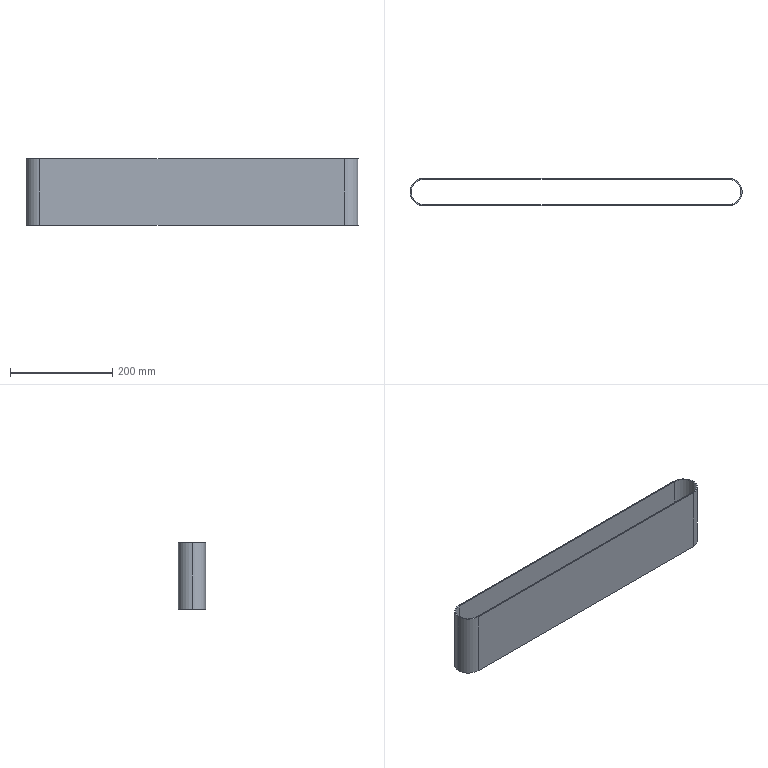Part | STEP file | Light green PVC conveyor belt 1346x129x2mm thick_antistatic | 1 solid | 12 faces | box 648.5 x 54 x 129 mm | volume 348910 mm3 | cylinder 6 | plane 6 | commonest cylinder face diameters 50 x3 54 x3
STEP:
#1=CARTESIAN_POINT('',(0.,0.,0.));
#2=DIRECTION('',(0.,0.,1.));
#3=DIRECTION('',(1.,0.,0.));
#4=AXIS2_PLACEMENT_3D('',#1,#2,#3);
#5=CARTESIAN_POINT('',(-297.25,25.,64.5));
#6=VERTEX_POINT('',#5);
#7=CARTESIAN_POINT('',(-297.25,25.,-64.5));
#8=VERTEX_POINT('',#7);
#9=CARTESIAN_POINT('',(-297.25,25.,64.5));
#10=DIRECTION('',(0.,0.,-1.));
#11=VECTOR('',#10,1.);
#12=LINE('',#9,#11);
#13=CARTESIAN_POINT('',(-297.25,0.,64.5));
#14=DIRECTION('',(0.,0.,-1.));
#15=DIRECTION('',(-1.,0.,0.));
#16=AXIS2_PLACEMENT_3D('',#13,#14,#15);
#17=CYLINDRICAL_SURFACE('',#16,25.);
#18=CARTESIAN_POINT('',(1.571,0.));
#19=DIRECTION('',(0.,1.));
#20=VECTOR('',#19,1.);
#21=LINE('',#18,#20);
#22=(GEOMETRIC_REPRESENTATION_CONTEXT(2)PARAMETRIC_REPRESENTATION_CONTEXT()REPRESENTATION_CONTEXT('',''));
#23=DEFINITIONAL_REPRESENTATION('',(#21),#22);
#24=PCURVE('',#17,#23);
#25=CARTESIAN_POINT('',(-297.25,25.,64.5));
#26=DIRECTION('',(0.,-1.,0.));
#27=DIRECTION('',(0.,0.,-1.));
#28=AXIS2_PLACEMENT_3D('',#25,#26,#27);
#29=PLANE('',#28);
#30=CARTESIAN_POINT('',(0.,0.));
#31=DIRECTION('',(1.,0.));
#32=VECTOR('',#31,1.);
#33=LINE('',#30,#32);
#34=(GEOMETRIC_REPRESENTATION_CONTEXT(2)PARAMETRIC_REPRESENTATION_CONTEXT()REPRESENTATION_CONTEXT('',''));
#35=DEFINITIONAL_REPRESENTATION('',(#33),#34);
#36=PCURVE('',#29,#35);
#37=SURFACE_CURVE('',#12,(#24,#36),.PCURVE_S1.);
#38=EDGE_CURVE('',#6,#8,#37,.T.);
#39=ORIENTED_EDGE('',*,*,#38,.T.);
#40=CARTESIAN_POINT('',(-322.25,0.,-64.5));
#41=VERTEX_POINT('',#40);
#42=CARTESIAN_POINT('',(-297.25,0.,-64.5));
#43=DIRECTION('',(0.,0.,1.));
#44=DIRECTION('',(1.,0.,0.));
#45=AXIS2_PLACEMENT_3D('',#42,#43,#44);
#46=CIRCLE('',#45,25.);
#47=CARTESIAN_POINT('',(3.142,129.));
#48=DIRECTION('',(-1.,0.));
#49=VECTOR('',#48,1.);
#50=LINE('',#47,#49);
#51=(GEOMETRIC_REPRESENTATION_CONTEXT(2)PARAMETRIC_REPRESENTATION_CONTEXT()REPRESENTATION_CONTEXT('',''));
#52=DEFINITIONAL_REPRESENTATION('',(#50),#51);
#53=PCURVE('',#17,#52);
#54=CARTESIAN_POINT('',(-297.25,0.,-64.5));
#55=DIRECTION('',(0.,0.,1.));
#56=DIRECTION('',(1.,0.,0.));
#57=AXIS2_PLACEMENT_3D('',#54,#55,#56);
#58=PLANE('',#57);
#59=CARTESIAN_POINT('',(0.,0.));
#60=DIRECTION('',(1.,0.));
#61=AXIS2_PLACEMENT_2D('',#59,#60);
#62=CIRCLE('',#61,25.);
#63=(GEOMETRIC_REPRESENTATION_CONTEXT(2)PARAMETRIC_REPRESENTATION_CONTEXT()REPRESENTATION_CONTEXT('',''));
#64=DEFINITIONAL_REPRESENTATION('',(#62),#63);
#65=PCURVE('',#58,#64);
#66=SURFACE_CURVE('',#46,(#53,#65),.PCURVE_S1.);
#67=EDGE_CURVE('',#8,#41,#66,.T.);
#68=ORIENTED_EDGE('',*,*,#67,.T.);
#69=CARTESIAN_POINT('',(-322.25,0.,64.5));
#70=VERTEX_POINT('',#69);
#71=CARTESIAN_POINT('',(-322.25,0.,64.5));
#72=DIRECTION('',(0.,0.,-1.));
#73=VECTOR('',#72,1.);
#74=LINE('',#71,#73);
#75=CARTESIAN_POINT('',(0.,0.));
#76=DIRECTION('',(0.,1.));
#77=VECTOR('',#76,1.);
#78=LINE('',#75,#77);
#79=(GEOMETRIC_REPRESENTATION_CONTEXT(2)PARAMETRIC_REPRESENTATION_CONTEXT()REPRESENTATION_CONTEXT('',''));
#80=DEFINITIONAL_REPRESENTATION('',(#78),#79);
#81=PCURVE('',#17,#80);
#82=CARTESIAN_POINT('',(-297.25,0.,64.5));
#83=DIRECTION('',(0.,0.,-1.));
#84=DIRECTION('',(-1.,0.,0.));
#85=AXIS2_PLACEMENT_3D('',#82,#83,#84);
#86=CYLINDRICAL_SURFACE('',#85,25.);
#87=CARTESIAN_POINT('',(6.283,0.));
#88=DIRECTION('',(0.,1.));
#89=VECTOR('',#88,1.);
#90=LINE('',#87,#89);
#91=(GEOMETRIC_REPRESENTATION_CONTEXT(2)PARAMETRIC_REPRESENTATION_CONTEXT()REPRESENTATION_CONTEXT('',''));
#92=DEFINITIONAL_REPRESENTATION('',(#90),#91);
#93=PCURVE('',#86,#92);
#94=SURFACE_CURVE('',#74,(#81,#93),.PCURVE_S1.);
#95=EDGE_CURVE('',#70,#41,#94,.T.);
#96=ORIENTED_EDGE('',*,*,#95,.F.);
#97=CARTESIAN_POINT('',(-297.25,0.,64.5));
#98=DIRECTION('',(0.,0.,1.));
#99=DIRECTION('',(1.,0.,0.));
#100=AXIS2_PLACEMENT_3D('',#97,#98,#99);
#101=CIRCLE('',#100,25.);
#102=CARTESIAN_POINT('',(3.142,0.));
#103=DIRECTION('',(-1.,0.));
#104=VECTOR('',#103,1.);
#105=LINE('',#102,#104);
#106=(GEOMETRIC_REPRESENTATION_CONTEXT(2)PARAMETRIC_REPRESENTATION_CONTEXT()REPRESENTATION_CONTEXT('',''));
#107=DEFINITIONAL_REPRESENTATION('',(#105),#106);
#108=PCURVE('',#17,#107);
#109=CARTESIAN_POINT('',(-297.25,0.,64.5));
#110=DIRECTION('',(0.,0.,1.));
#111=DIRECTION('',(1.,0.,0.));
#112=AXIS2_PLACEMENT_3D('',#109,#110,#111);
#113=PLANE('',#112);
#114=CARTESIAN_POINT('',(0.,0.));
#115=DIRECTION('',(1.,0.));
#116=AXIS2_PLACEMENT_2D('',#114,#115);
#117=CIRCLE('',#116,25.);
#118=(GEOMETRIC_REPRESENTATION_CONTEXT(2)PARAMETRIC_REPRESENTATION_CONTEXT()REPRESENTATION_CONTEXT('',''));
#119=DEFINITIONAL_REPRESENTATION('',(#117),#118);
#120=PCURVE('',#113,#119);
#121=SURFACE_CURVE('',#101,(#108,#120),.PCURVE_S1.);
#122=EDGE_CURVE('',#6,#70,#121,.T.);
#123=ORIENTED_EDGE('',*,*,#122,.F.);
#124=EDGE_LOOP('',(#39,#68,#96,#123));
#125=FACE_BOUND('',#124,.F.);
#126=ADVANCED_FACE('',(#125),#17,.F.);
#127=CARTESIAN_POINT('',(-324.25,0.,64.5));
#128=VERTEX_POINT('',#127);
#129=CARTESIAN_POINT('',(-297.25,-27.,64.5));
#130=VERTEX_POINT('',#129);
#131=CARTESIAN_POINT('',(-297.25,0.,64.5));
#132=DIRECTION('',(0.,0.,1.));
#133=DIRECTION('',(1.,0.,0.));
#134=AXIS2_PLACEMENT_3D('',#131,#132,#133);
#135=CIRCLE('',#134,27.);
#136=CARTESIAN_POINT('',(-297.25,0.,64.5));
#137=DIRECTION('',(0.,0.,-1.));
#138=DIRECTION('',(-1.,0.,0.));
#139=AXIS2_PLACEMENT_3D('',#136,#137,#138);
#140=CYLINDRICAL_SURFACE('',#139,27.);
#141=CARTESIAN_POINT('',(9.425,0.));
#142=DIRECTION('',(-1.,0.));
#143=VECTOR('',#142,1.);
#144=LINE('',#141,#143);
#145=(GEOMETRIC_REPRESENTATION_CONTEXT(2)PARAMETRIC_REPRESENTATION_CONTEXT()REPRESENTATION_CONTEXT('',''));
#146=DEFINITIONAL_REPRESENTATION('',(#144),#145);
#147=PCURVE('',#140,#146);
#148=CARTESIAN_POINT('',(0.,0.));
#149=DIRECTION('',(1.,0.));
#150=AXIS2_PLACEMENT_2D('',#148,#149);
#151=CIRCLE('',#150,27.);
#152=(GEOMETRIC_REPRESENTATION_CONTEXT(2)PARAMETRIC_REPRESENTATION_CONTEXT()REPRESENTATION_CONTEXT('',''));
#153=DEFINITIONAL_REPRESENTATION('',(#151),#152);
#154=PCURVE('',#113,#153);
#155=SURFACE_CURVE('',#135,(#147,#154),.PCURVE_S1.);
#156=EDGE_CURVE('',#128,#130,#155,.T.);
#157=ORIENTED_EDGE('',*,*,#156,.F.);
#158=CARTESIAN_POINT('',(-324.25,0.,-64.5));
#159=VERTEX_POINT('',#158);
#160=CARTESIAN_POINT('',(-324.25,0.,64.5));
#161=DIRECTION('',(0.,0.,-1.));
#162=VECTOR('',#161,1.);
#163=LINE('',#160,#162);
#164=CARTESIAN_POINT('',(6.283,0.));
#165=DIRECTION('',(0.,1.));
#166=VECTOR('',#165,1.);
#167=LINE('',#164,#166);
#168=(GEOMETRIC_REPRESENTATION_CONTEXT(2)PARAMETRIC_REPRESENTATION_CONTEXT()REPRESENTATION_CONTEXT('',''));
#169=DEFINITIONAL_REPRESENTATION('',(#167),#168);
#170=PCURVE('',#140,#169);
#171=CARTESIAN_POINT('',(-297.25,0.,64.5));
#172=DIRECTION('',(0.,0.,-1.));
#173=DIRECTION('',(-1.,0.,0.));
#174=AXIS2_PLACEMENT_3D('',#171,#172,#173);
#175=CYLINDRICAL_SURFACE('',#174,27.);
#176=CARTESIAN_POINT('',(0.,0.));
#177=DIRECTION('',(0.,1.));
#178=VECTOR('',#177,1.);
#179=LINE('',#176,#178);
#180=(GEOMETRIC_REPRESENTATION_CONTEXT(2)PARAMETRIC_REPRESENTATION_CONTEXT()REPRESENTATION_CONTEXT('',''));
#181=DEFINITIONAL_REPRESENTATION('',(#179),#180);
#182=PCURVE('',#175,#181);
#183=SURFACE_CURVE('',#163,(#170,#182),.PCURVE_S1.);
#184=EDGE_CURVE('',#128,#159,#183,.T.);
#185=ORIENTED_EDGE('',*,*,#184,.T.);
#186=CARTESIAN_POINT('',(-297.25,-27.,-64.5));
#187=VERTEX_POINT('',#186);
#188=CARTESIAN_POINT('',(-297.25,0.,-64.5));
#189=DIRECTION('',(0.,0.,1.));
#190=DIRECTION('',(1.,0.,0.));
#191=AXIS2_PLACEMENT_3D('',#188,#189,#190);
#192=CIRCLE('',#191,27.);
#193=CARTESIAN_POINT('',(9.425,129.));
#194=DIRECTION('',(-1.,0.));
#195=VECTOR('',#194,1.);
#196=LINE('',#193,#195);
#197=(GEOMETRIC_REPRESENTATION_CONTEXT(2)PARAMETRIC_REPRESENTATION_CONTEXT()REPRESENTATION_CONTEXT('',''));
#198=DEFINITIONAL_REPRESENTATION('',(#196),#197);
#199=PCURVE('',#140,#198);
#200=CARTESIAN_POINT('',(0.,0.));
#201=DIRECTION('',(1.,0.));
#202=AXIS2_PLACEMENT_2D('',#200,#201);
#203=CIRCLE('',#202,27.);
#204=(GEOMETRIC_REPRESENTATION_CONTEXT(2)PARAMETRIC_REPRESENTATION_CONTEXT()REPRESENTATION_CONTEXT('',''));
#205=DEFINITIONAL_REPRESENTATION('',(#203),#204);
#206=PCURVE('',#58,#205);
#207=SURFACE_CURVE('',#192,(#199,#206),.PCURVE_S1.);
#208=EDGE_CURVE('',#159,#187,#207,.T.);
#209=ORIENTED_EDGE('',*,*,#208,.T.);
#210=CARTESIAN_POINT('',(-297.25,-27.,64.5));
#211=DIRECTION('',(0.,0.,-1.));
#212=VECTOR('',#211,1.);
#213=LINE('',#210,#212);
#214=CARTESIAN_POINT('',(4.712,0.));
#215=DIRECTION('',(0.,1.));
#216=VECTOR('',#215,1.);
#217=LINE('',#214,#216);
#218=(GEOMETRIC_REPRESENTATION_CONTEXT(2)PARAMETRIC_REPRESENTATION_CONTEXT()REPRESENTATION_CONTEXT('',''));
#219=DEFINITIONAL_REPRESENTATION('',(#217),#218);
#220=PCURVE('',#140,#219);
#221=CARTESIAN_POINT('',(-297.25,-27.,64.5));
#222=DIRECTION('',(0.,1.,0.));
#223=DIRECTION('',(0.,0.,1.));
#224=AXIS2_PLACEMENT_3D('',#221,#222,#223);
#225=PLANE('',#224);
#226=CARTESIAN_POINT('',(0.,0.));
#227=DIRECTION('',(-1.,0.));
#228=VECTOR('',#227,1.);
#229=LINE('',#226,#228);
#230=(GEOMETRIC_REPRESENTATION_CONTEXT(2)PARAMETRIC_REPRESENTATION_CONTEXT()REPRESENTATION_CONTEXT('',''));
#231=DEFINITIONAL_REPRESENTATION('',(#229),#230);
#232=PCURVE('',#225,#231);
#233=SURFACE_CURVE('',#213,(#220,#232),.PCURVE_S1.);
#234=EDGE_CURVE('',#130,#187,#233,.T.);
#235=ORIENTED_EDGE('',*,*,#234,.F.);
#236=EDGE_LOOP('',(#157,#185,#209,#235));
#237=FACE_BOUND('',#236,.T.);
#238=ADVANCED_FACE('',(#237),#140,.T.);
#239=CARTESIAN_POINT('',(-297.25,27.,64.5));
#240=VERTEX_POINT('',#239);
#241=CARTESIAN_POINT('',(-297.25,0.,64.5));
#242=DIRECTION('',(0.,0.,1.));
#243=DIRECTION('',(1.,0.,0.));
#244=AXIS2_PLACEMENT_3D('',#241,#242,#243);
#245=CIRCLE('',#244,27.);
#246=CARTESIAN_POINT('',(0.,0.));
#247=DIRECTION('',(1.,0.));
#248=AXIS2_PLACEMENT_2D('',#246,#247);
#249=CIRCLE('',#248,27.);
#250=(GEOMETRIC_REPRESENTATION_CONTEXT(2)PARAMETRIC_REPRESENTATION_CONTEXT()REPRESENTATION_CONTEXT('',''));
#251=DEFINITIONAL_REPRESENTATION('',(#249),#250);
#252=PCURVE('',#113,#251);
#253=CARTESIAN_POINT('',(3.142,0.));
#254=DIRECTION('',(-1.,0.));
#255=VECTOR('',#254,1.);
#256=LINE('',#253,#255);
#257=(GEOMETRIC_REPRESENTATION_CONTEXT(2)PARAMETRIC_REPRESENTATION_CONTEXT()REPRESENTATION_CONTEXT('',''));
#258=DEFINITIONAL_REPRESENTATION('',(#256),#257);
#259=PCURVE('',#175,#258);
#260=SURFACE_CURVE('',#245,(#252,#259),.PCURVE_S1.);
#261=EDGE_CURVE('',#240,#128,#260,.T.);
#262=ORIENTED_EDGE('',*,*,#261,.T.);
#263=ORIENTED_EDGE('',*,*,#156,.T.);
#264=CARTESIAN_POINT('',(297.25,-27.,64.5));
#265=VERTEX_POINT('',#264);
#266=CARTESIAN_POINT('',(-297.25,-27.,64.5));
#267=DIRECTION('',(1.,0.,0.));
#268=VECTOR('',#267,1.);
#269=LINE('',#266,#268);
#270=CARTESIAN_POINT('',(0.,-27.));
#271=DIRECTION('',(1.,0.));
#272=VECTOR('',#271,1.);
#273=LINE('',#270,#272);
#274=(GEOMETRIC_REPRESENTATION_CONTEXT(2)PARAMETRIC_REPRESENTATION_CONTEXT()REPRESENTATION_CONTEXT('',''));
#275=DEFINITIONAL_REPRESENTATION('',(#273),#274);
#276=PCURVE('',#113,#275);
#277=CARTESIAN_POINT('',(0.,0.));
#278=DIRECTION('',(0.,1.));
#279=VECTOR('',#278,1.);
#280=LINE('',#277,#279);
#281=(GEOMETRIC_REPRESENTATION_CONTEXT(2)PARAMETRIC_REPRESENTATION_CONTEXT()REPRESENTATION_CONTEXT('',''));
#282=DEFINITIONAL_REPRESENTATION('',(#280),#281);
#283=PCURVE('',#225,#282);
#284=SURFACE_CURVE('',#269,(#276,#283),.PCURVE_S1.);
#285=EDGE_CURVE('',#130,#265,#284,.T.);
#286=ORIENTED_EDGE('',*,*,#285,.T.);
#287=CARTESIAN_POINT('',(297.25,27.,64.5));
#288=VERTEX_POINT('',#287);
#289=CARTESIAN_POINT('',(297.25,0.,64.5));
#290=DIRECTION('',(0.,0.,1.));
#291=DIRECTION('',(1.,0.,0.));
#292=AXIS2_PLACEMENT_3D('',#289,#290,#291);
#293=CIRCLE('',#292,27.);
#294=CARTESIAN_POINT('',(594.5,0.));
#295=DIRECTION('',(1.,0.));
#296=AXIS2_PLACEMENT_2D('',#294,#295);
#297=CIRCLE('',#296,27.);
#298=(GEOMETRIC_REPRESENTATION_CONTEXT(2)PARAMETRIC_REPRESENTATION_CONTEXT()REPRESENTATION_CONTEXT('',''));
#299=DEFINITIONAL_REPRESENTATION('',(#297),#298);
#300=PCURVE('',#113,#299);
#301=CARTESIAN_POINT('',(297.25,0.,64.5));
#302=DIRECTION('',(0.,0.,-1.));
#303=DIRECTION('',(-1.,0.,0.));
#304=AXIS2_PLACEMENT_3D('',#301,#302,#303);
#305=CYLINDRICAL_SURFACE('',#304,27.);
#306=CARTESIAN_POINT('',(9.425,0.));
#307=DIRECTION('',(-1.,0.));
#308=VECTOR('',#307,1.);
#309=LINE('',#306,#308);
#310=(GEOMETRIC_REPRESENTATION_CONTEXT(2)PARAMETRIC_REPRESENTATION_CONTEXT()REPRESENTATION_CONTEXT('',''));
#311=DEFINITIONAL_REPRESENTATION('',(#309),#310);
#312=PCURVE('',#305,#311);
#313=SURFACE_CURVE('',#293,(#300,#312),.PCURVE_S1.);
#314=EDGE_CURVE('',#265,#288,#313,.T.);
#315=ORIENTED_EDGE('',*,*,#314,.T.);
#316=CARTESIAN_POINT('',(-297.25,27.,64.5));
#317=DIRECTION('',(-1.,0.,0.));
#318=VECTOR('',#317,1.);
#319=LINE('',#316,#318);
#320=CARTESIAN_POINT('',(0.,27.));
#321=DIRECTION('',(-1.,0.));
#322=VECTOR('',#321,1.);
#323=LINE('',#320,#322);
#324=(GEOMETRIC_REPRESENTATION_CONTEXT(2)PARAMETRIC_REPRESENTATION_CONTEXT()REPRESENTATION_CONTEXT('',''));
#325=DEFINITIONAL_REPRESENTATION('',(#323),#324);
#326=PCURVE('',#113,#325);
#327=CARTESIAN_POINT('',(-297.25,27.,64.5));
#328=DIRECTION('',(0.,-1.,0.));
#329=DIRECTION('',(0.,0.,-1.));
#330=AXIS2_PLACEMENT_3D('',#327,#328,#329);
#331=PLANE('',#330);
#332=CARTESIAN_POINT('',(0.,0.));
#333=DIRECTION('',(0.,-1.));
#334=VECTOR('',#333,1.);
#335=LINE('',#332,#334);
#336=(GEOMETRIC_REPRESENTATION_CONTEXT(2)PARAMETRIC_REPRESENTATION_CONTEXT()REPRESENTATION_CONTEXT('',''));
#337=DEFINITIONAL_REPRESENTATION('',(#335),#336);
#338=PCURVE('',#331,#337);
#339=SURFACE_CURVE('',#319,(#326,#338),.PCURVE_S1.);
#340=EDGE_CURVE('',#288,#240,#339,.T.);
#341=ORIENTED_EDGE('',*,*,#340,.T.);
#342=EDGE_LOOP('',(#262,#263,#286,#315,#341));
#343=FACE_BOUND('',#342,.T.);
#344=CARTESIAN_POINT('',(-297.25,-25.,64.5));
#345=VERTEX_POINT('',#344);
#346=CARTESIAN_POINT('',(297.25,-25.,64.5));
#347=VERTEX_POINT('',#346);
#348=CARTESIAN_POINT('',(-297.25,-25.,64.5));
#349=DIRECTION('',(1.,0.,0.));
#350=VECTOR('',#349,1.);
#351=LINE('',#348,#350);
#352=CARTESIAN_POINT('',(0.,-25.));
#353=DIRECTION('',(1.,0.));
#354=VECTOR('',#353,1.);
#355=LINE('',#352,#354);
#356=(GEOMETRIC_REPRESENTATION_CONTEXT(2)PARAMETRIC_REPRESENTATION_CONTEXT()REPRESENTATION_CONTEXT('',''));
#357=DEFINITIONAL_REPRESENTATION('',(#355),#356);
#358=PCURVE('',#113,#357);
#359=CARTESIAN_POINT('',(-297.25,-25.,64.5));
#360=DIRECTION('',(0.,1.,0.));
#361=DIRECTION('',(0.,0.,1.));
#362=AXIS2_PLACEMENT_3D('',#359,#360,#361);
#363=PLANE('',#362);
#364=CARTESIAN_POINT('',(0.,0.));
#365=DIRECTION('',(0.,1.));
#366=VECTOR('',#365,1.);
#367=LINE('',#364,#366);
#368=(GEOMETRIC_REPRESENTATION_CONTEXT(2)PARAMETRIC_REPRESENTATION_CONTEXT()REPRESENTATION_CONTEXT('',''));
#369=DEFINITIONAL_REPRESENTATION('',(#367),#368);
#370=PCURVE('',#363,#369);
#371=SURFACE_CURVE('',#351,(#358,#370),.PCURVE_S1.);
#372=EDGE_CURVE('',#345,#347,#371,.T.);
#373=ORIENTED_EDGE('',*,*,#372,.F.);
#374=CARTESIAN_POINT('',(-297.25,0.,64.5));
#375=DIRECTION('',(0.,0.,1.));
#376=DIRECTION('',(1.,0.,0.));
#377=AXIS2_PLACEMENT_3D('',#374,#375,#376);
#378=CIRCLE('',#377,25.);
#379=CARTESIAN_POINT('',(0.,0.));
#380=DIRECTION('',(1.,0.));
#381=AXIS2_PLACEMENT_2D('',#379,#380);
#382=CIRCLE('',#381,25.);
#383=(GEOMETRIC_REPRESENTATION_CONTEXT(2)PARAMETRIC_REPRESENTATION_CONTEXT()REPRESENTATION_CONTEXT('',''));
#384=DEFINITIONAL_REPRESENTATION('',(#382),#383);
#385=PCURVE('',#113,#384);
#386=CARTESIAN_POINT('',(9.425,0.));
#387=DIRECTION('',(-1.,0.));
#388=VECTOR('',#387,1.);
#389=LINE('',#386,#388);
#390=(GEOMETRIC_REPRESENTATION_CONTEXT(2)PARAMETRIC_REPRESENTATION_CONTEXT()REPRESENTATION_CONTEXT('',''));
#391=DEFINITIONAL_REPRESENTATION('',(#389),#390);
#392=PCURVE('',#86,#391);
#393=SURFACE_CURVE('',#378,(#385,#392),.PCURVE_S1.);
#394=EDGE_CURVE('',#70,#345,#393,.T.);
#395=ORIENTED_EDGE('',*,*,#394,.F.);
#396=ORIENTED_EDGE('',*,*,#122,.F.);
#397=CARTESIAN_POINT('',(297.25,25.,64.5));
#398=VERTEX_POINT('',#397);
#399=CARTESIAN_POINT('',(-297.25,25.,64.5));
#400=DIRECTION('',(-1.,0.,0.));
#401=VECTOR('',#400,1.);
#402=LINE('',#399,#401);
#403=CARTESIAN_POINT('',(0.,25.));
#404=DIRECTION('',(-1.,0.));
#405=VECTOR('',#404,1.);
#406=LINE('',#403,#405);
#407=(GEOMETRIC_REPRESENTATION_CONTEXT(2)PARAMETRIC_REPRESENTATION_CONTEXT()REPRESENTATION_CONTEXT('',''));
#408=DEFINITIONAL_REPRESENTATION('',(#406),#407);
#409=PCURVE('',#113,#408);
#410=CARTESIAN_POINT('',(0.,0.));
#411=DIRECTION('',(0.,-1.));
#412=VECTOR('',#411,1.);
#413=LINE('',#410,#412);
#414=(GEOMETRIC_REPRESENTATION_CONTEXT(2)PARAMETRIC_REPRESENTATION_CONTEXT()REPRESENTATION_CONTEXT('',''));
#415=DEFINITIONAL_REPRESENTATION('',(#413),#414);
#416=PCURVE('',#29,#415);
#417=SURFACE_CURVE('',#402,(#409,#416),.PCURVE_S1.);
#418=EDGE_CURVE('',#398,#6,#417,.T.);
#419=ORIENTED_EDGE('',*,*,#418,.F.);
#420=CARTESIAN_POINT('',(297.25,0.,64.5));
#421=DIRECTION('',(0.,0.,1.));
#422=DIRECTION('',(1.,0.,0.));
#423=AXIS2_PLACEMENT_3D('',#420,#421,#422);
#424=CIRCLE('',#423,25.);
#425=CARTESIAN_POINT('',(594.5,0.));
#426=DIRECTION('',(1.,0.));
#427=AXIS2_PLACEMENT_2D('',#425,#426);
#428=CIRCLE('',#427,25.);
#429=(GEOMETRIC_REPRESENTATION_CONTEXT(2)PARAMETRIC_REPRESENTATION_CONTEXT()REPRESENTATION_CONTEXT('',''));
#430=DEFINITIONAL_REPRESENTATION('',(#428),#429);
#431=PCURVE('',#113,#430);
#432=CARTESIAN_POINT('',(297.25,0.,64.5));
#433=DIRECTION('',(0.,0.,-1.));
#434=DIRECTION('',(-1.,0.,0.));
#435=AXIS2_PLACEMENT_3D('',#432,#433,#434);
#436=CYLINDRICAL_SURFACE('',#435,25.);
#437=CARTESIAN_POINT('',(9.425,0.));
#438=DIRECTION('',(-1.,0.));
#439=VECTOR('',#438,1.);
#440=LINE('',#437,#439);
#441=(GEOMETRIC_REPRESENTATION_CONTEXT(2)PARAMETRIC_REPRESENTATION_CONTEXT()REPRESENTATION_CONTEXT('',''));
#442=DEFINITIONAL_REPRESENTATION('',(#440),#441);
#443=PCURVE('',#436,#442);
#444=SURFACE_CURVE('',#424,(#431,#443),.PCURVE_S1.);
#445=EDGE_CURVE('',#347,#398,#444,.T.);
#446=ORIENTED_EDGE('',*,*,#445,.F.);
#447=EDGE_LOOP('',(#373,#395,#396,#419,#446));
#448=FACE_BOUND('',#447,.T.);
#449=ADVANCED_FACE('',(#343,#448),#113,.T.);
#450=CARTESIAN_POINT('',(-297.25,27.,-64.5));
#451=VERTEX_POINT('',#450);
#452=CARTESIAN_POINT('',(-297.25,0.,-64.5));
#453=DIRECTION('',(0.,0.,1.));
#454=DIRECTION('',(1.,0.,0.));
#455=AXIS2_PLACEMENT_3D('',#452,#453,#454);
#456=CIRCLE('',#455,27.);
#457=CARTESIAN_POINT('',(0.,0.));
#458=DIRECTION('',(1.,0.));
#459=AXIS2_PLACEMENT_2D('',#457,#458);
#460=CIRCLE('',#459,27.);
#461=(GEOMETRIC_REPRESENTATION_CONTEXT(2)PARAMETRIC_REPRESENTATION_CONTEXT()REPRESENTATION_CONTEXT('',''));
#462=DEFINITIONAL_REPRESENTATION('',(#460),#461);
#463=PCURVE('',#58,#462);
#464=CARTESIAN_POINT('',(3.142,129.));
#465=DIRECTION('',(-1.,0.));
#466=VECTOR('',#465,1.);
#467=LINE('',#464,#466);
#468=(GEOMETRIC_REPRESENTATION_CONTEXT(2)PARAMETRIC_REPRESENTATION_CONTEXT()REPRESENTATION_CONTEXT('',''));
#469=DEFINITIONAL_REPRESENTATION('',(#467),#468);
#470=PCURVE('',#175,#469);
#471=SURFACE_CURVE('',#456,(#463,#470),.PCURVE_S1.);
#472=EDGE_CURVE('',#451,#159,#471,.T.);
#473=ORIENTED_EDGE('',*,*,#472,.F.);
#474=CARTESIAN_POINT('',(297.25,27.,-64.5));
#475=VERTEX_POINT('',#474);
#476=CARTESIAN_POINT('',(-297.25,27.,-64.5));
#477=DIRECTION('',(-1.,0.,0.));
#478=VECTOR('',#477,1.);
#479=LINE('',#476,#478);
#480=CARTESIAN_POINT('',(0.,27.));
#481=DIRECTION('',(-1.,0.));
#482=VECTOR('',#481,1.);
#483=LINE('',#480,#482);
#484=(GEOMETRIC_REPRESENTATION_CONTEXT(2)PARAMETRIC_REPRESENTATION_CONTEXT()REPRESENTATION_CONTEXT('',''));
#485=DEFINITIONAL_REPRESENTATION('',(#483),#484);
#486=PCURVE('',#58,#485);
#487=CARTESIAN_POINT('',(129.,0.));
#488=DIRECTION('',(0.,-1.));
#489=VECTOR('',#488,1.);
#490=LINE('',#487,#489);
#491=(GEOMETRIC_REPRESENTATION_CONTEXT(2)PARAMETRIC_REPRESENTATION_CONTEXT()REPRESENTATION_CONTEXT('',''));
#492=DEFINITIONAL_REPRESENTATION('',(#490),#491);
#493=PCURVE('',#331,#492);
#494=SURFACE_CURVE('',#479,(#486,#493),.PCURVE_S1.);
#495=EDGE_CURVE('',#475,#451,#494,.T.);
#496=ORIENTED_EDGE('',*,*,#495,.F.);
#497=CARTESIAN_POINT('',(297.25,-27.,-64.5));
#498=VERTEX_POINT('',#497);
#499=CARTESIAN_POINT('',(297.25,0.,-64.5));
#500=DIRECTION('',(0.,0.,1.));
#501=DIRECTION('',(1.,0.,0.));
#502=AXIS2_PLACEMENT_3D('',#499,#500,#501);
#503=CIRCLE('',#502,27.);
#504=CARTESIAN_POINT('',(594.5,0.));
#505=DIRECTION('',(1.,0.));
#506=AXIS2_PLACEMENT_2D('',#504,#505);
#507=CIRCLE('',#506,27.);
#508=(GEOMETRIC_REPRESENTATION_CONTEXT(2)PARAMETRIC_REPRESENTATION_CONTEXT()REPRESENTATION_CONTEXT('',''));
#509=DEFINITIONAL_REPRESENTATION('',(#507),#508);
#510=PCURVE('',#58,#509);
#511=CARTESIAN_POINT('',(9.425,129.));
#512=DIRECTION('',(-1.,0.));
#513=VECTOR('',#512,1.);
#514=LINE('',#511,#513);
#515=(GEOMETRIC_REPRESENTATION_CONTEXT(2)PARAMETRIC_REPRESENTATION_CONTEXT()REPRESENTATION_CONTEXT('',''));
#516=DEFINITIONAL_REPRESENTATION('',(#514),#515);
#517=PCURVE('',#305,#516);
#518=SURFACE_CURVE('',#503,(#510,#517),.PCURVE_S1.);
#519=EDGE_CURVE('',#498,#475,#518,.T.);
#520=ORIENTED_EDGE('',*,*,#519,.F.);
#521=CARTESIAN_POINT('',(-297.25,-27.,-64.5));
#522=DIRECTION('',(1.,0.,0.));
#523=VECTOR('',#522,1.);
#524=LINE('',#521,#523);
#525=CARTESIAN_POINT('',(0.,-27.));
#526=DIRECTION('',(1.,0.));
#527=VECTOR('',#526,1.);
#528=LINE('',#525,#527);
#529=(GEOMETRIC_REPRESENTATION_CONTEXT(2)PARAMETRIC_REPRESENTATION_CONTEXT()REPRESENTATION_CONTEXT('',''));
#530=DEFINITIONAL_REPRESENTATION('',(#528),#529);
#531=PCURVE('',#58,#530);
#532=CARTESIAN_POINT('',(-129.,0.));
#533=DIRECTION('',(0.,1.));
#534=VECTOR('',#533,1.);
#535=LINE('',#532,#534);
#536=(GEOMETRIC_REPRESENTATION_CONTEXT(2)PARAMETRIC_REPRESENTATION_CONTEXT()REPRESENTATION_CONTEXT('',''));
#537=DEFINITIONAL_REPRESENTATION('',(#535),#536);
#538=PCURVE('',#225,#537);
#539=SURFACE_CURVE('',#524,(#531,#538),.PCURVE_S1.);
#540=EDGE_CURVE('',#187,#498,#539,.T.);
#541=ORIENTED_EDGE('',*,*,#540,.F.);
#542=ORIENTED_EDGE('',*,*,#208,.F.);
#543=EDGE_LOOP('',(#473,#496,#520,#541,#542));
#544=FACE_BOUND('',#543,.T.);
#545=ORIENTED_EDGE('',*,*,#67,.T.);
#546=CARTESIAN_POINT('',(-297.25,-25.,-64.5));
#547=VERTEX_POINT('',#546);
#548=CARTESIAN_POINT('',(-297.25,0.,-64.5));
#549=DIRECTION('',(0.,0.,1.));
#550=DIRECTION('',(1.,0.,0.));
#551=AXIS2_PLACEMENT_3D('',#548,#549,#550);
#552=CIRCLE('',#551,25.);
#553=CARTESIAN_POINT('',(0.,0.));
#554=DIRECTION('',(1.,0.));
#555=AXIS2_PLACEMENT_2D('',#553,#554);
#556=CIRCLE('',#555,25.);
#557=(GEOMETRIC_REPRESENTATION_CONTEXT(2)PARAMETRIC_REPRESENTATION_CONTEXT()REPRESENTATION_CONTEXT('',''));
#558=DEFINITIONAL_REPRESENTATION('',(#556),#557);
#559=PCURVE('',#58,#558);
#560=CARTESIAN_POINT('',(9.425,129.));
#561=DIRECTION('',(-1.,0.));
#562=VECTOR('',#561,1.);
#563=LINE('',#560,#562);
#564=(GEOMETRIC_REPRESENTATION_CONTEXT(2)PARAMETRIC_REPRESENTATION_CONTEXT()REPRESENTATION_CONTEXT('',''));
#565=DEFINITIONAL_REPRESENTATION('',(#563),#564);
#566=PCURVE('',#86,#565);
#567=SURFACE_CURVE('',#552,(#559,#566),.PCURVE_S1.);
#568=EDGE_CURVE('',#41,#547,#567,.T.);
#569=ORIENTED_EDGE('',*,*,#568,.T.);
#570=CARTESIAN_POINT('',(297.25,-25.,-64.5));
#571=VERTEX_POINT('',#570);
#572=CARTESIAN_POINT('',(-297.25,-25.,-64.5));
#573=DIRECTION('',(1.,0.,0.));
#574=VECTOR('',#573,1.);
#575=LINE('',#572,#574);
#576=CARTESIAN_POINT('',(0.,-25.));
#577=DIRECTION('',(1.,0.));
#578=VECTOR('',#577,1.);
#579=LINE('',#576,#578);
#580=(GEOMETRIC_REPRESENTATION_CONTEXT(2)PARAMETRIC_REPRESENTATION_CONTEXT()REPRESENTATION_CONTEXT('',''));
#581=DEFINITIONAL_REPRESENTATION('',(#579),#580);
#582=PCURVE('',#58,#581);
#583=CARTESIAN_POINT('',(-129.,0.));
#584=DIRECTION('',(0.,1.));
#585=VECTOR('',#584,1.);
#586=LINE('',#583,#585);
#587=(GEOMETRIC_REPRESENTATION_CONTEXT(2)PARAMETRIC_REPRESENTATION_CONTEXT()REPRESENTATION_CONTEXT('',''));
#588=DEFINITIONAL_REPRESENTATION('',(#586),#587);
#589=PCURVE('',#363,#588);
#590=SURFACE_CURVE('',#575,(#582,#589),.PCURVE_S1.);
#591=EDGE_CURVE('',#547,#571,#590,.T.);
#592=ORIENTED_EDGE('',*,*,#591,.T.);
#593=CARTESIAN_POINT('',(297.25,25.,-64.5));
#594=VERTEX_POINT('',#593);
#595=CARTESIAN_POINT('',(297.25,0.,-64.5));
#596=DIRECTION('',(0.,0.,1.));
#597=DIRECTION('',(1.,0.,0.));
#598=AXIS2_PLACEMENT_3D('',#595,#596,#597);
#599=CIRCLE('',#598,25.);
#600=CARTESIAN_POINT('',(594.5,0.));
#601=DIRECTION('',(1.,0.));
#602=AXIS2_PLACEMENT_2D('',#600,#601);
#603=CIRCLE('',#602,25.);
#604=(GEOMETRIC_REPRESENTATION_CONTEXT(2)PARAMETRIC_REPRESENTATION_CONTEXT()REPRESENTATION_CONTEXT('',''));
#605=DEFINITIONAL_REPRESENTATION('',(#603),#604);
#606=PCURVE('',#58,#605);
#607=CARTESIAN_POINT('',(9.425,129.));
#608=DIRECTION('',(-1.,0.));
#609=VECTOR('',#608,1.);
#610=LINE('',#607,#609);
#611=(GEOMETRIC_REPRESENTATION_CONTEXT(2)PARAMETRIC_REPRESENTATION_CONTEXT()REPRESENTATION_CONTEXT('',''));
#612=DEFINITIONAL_REPRESENTATION('',(#610),#611);
#613=PCURVE('',#436,#612);
#614=SURFACE_CURVE('',#599,(#606,#613),.PCURVE_S1.);
#615=EDGE_CURVE('',#571,#594,#614,.T.);
#616=ORIENTED_EDGE('',*,*,#615,.T.);
#617=CARTESIAN_POINT('',(-297.25,25.,-64.5));
#618=DIRECTION('',(-1.,0.,0.));
#619=VECTOR('',#618,1.);
#620=LINE('',#617,#619);
#621=CARTESIAN_POINT('',(0.,25.));
#622=DIRECTION('',(-1.,0.));
#623=VECTOR('',#622,1.);
#624=LINE('',#621,#623);
#625=(GEOMETRIC_REPRESENTATION_CONTEXT(2)PARAMETRIC_REPRESENTATION_CONTEXT()REPRESENTATION_CONTEXT('',''));
#626=DEFINITIONAL_REPRESENTATION('',(#624),#625);
#627=PCURVE('',#58,#626);
#628=CARTESIAN_POINT('',(129.,0.));
#629=DIRECTION('',(0.,-1.));
#630=VECTOR('',#629,1.);
#631=LINE('',#628,#630);
#632=(GEOMETRIC_REPRESENTATION_CONTEXT(2)PARAMETRIC_REPRESENTATION_CONTEXT()REPRESENTATION_CONTEXT('',''));
#633=DEFINITIONAL_REPRESENTATION('',(#631),#632);
#634=PCURVE('',#29,#633);
#635=SURFACE_CURVE('',#620,(#627,#634),.PCURVE_S1.);
#636=EDGE_CURVE('',#594,#8,#635,.T.);
#637=ORIENTED_EDGE('',*,*,#636,.T.);
#638=EDGE_LOOP('',(#545,#569,#592,#616,#637));
#639=FACE_BOUND('',#638,.T.);
#640=ADVANCED_FACE('',(#544,#639),#58,.F.);
#641=ORIENTED_EDGE('',*,*,#184,.F.);
#642=ORIENTED_EDGE('',*,*,#261,.F.);
#643=CARTESIAN_POINT('',(-297.25,27.,64.5));
#644=DIRECTION('',(0.,0.,-1.));
#645=VECTOR('',#644,1.);
#646=LINE('',#643,#645);
#647=CARTESIAN_POINT('',(1.571,0.));
#648=DIRECTION('',(0.,1.));
#649=VECTOR('',#648,1.);
#650=LINE('',#647,#649);
#651=(GEOMETRIC_REPRESENTATION_CONTEXT(2)PARAMETRIC_REPRESENTATION_CONTEXT()REPRESENTATION_CONTEXT('',''));
#652=DEFINITIONAL_REPRESENTATION('',(#650),#651);
#653=PCURVE('',#175,#652);
#654=CARTESIAN_POINT('',(0.,0.));
#655=DIRECTION('',(1.,0.));
#656=VECTOR('',#655,1.);
#657=LINE('',#654,#656);
#658=(GEOMETRIC_REPRESENTATION_CONTEXT(2)PARAMETRIC_REPRESENTATION_CONTEXT()REPRESENTATION_CONTEXT('',''));
#659=DEFINITIONAL_REPRESENTATION('',(#657),#658);
#660=PCURVE('',#331,#659);
#661=SURFACE_CURVE('',#646,(#653,#660),.PCURVE_S1.);
#662=EDGE_CURVE('',#240,#451,#661,.T.);
#663=ORIENTED_EDGE('',*,*,#662,.T.);
#664=ORIENTED_EDGE('',*,*,#472,.T.);
#665=EDGE_LOOP('',(#641,#642,#663,#664));
#666=FACE_BOUND('',#665,.T.);
#667=ADVANCED_FACE('',(#666),#175,.T.);
#668=ORIENTED_EDGE('',*,*,#540,.T.);
#669=CARTESIAN_POINT('',(297.25,-27.,64.5));
#670=DIRECTION('',(0.,0.,-1.));
#671=VECTOR('',#670,1.);
#672=LINE('',#669,#671);
#673=CARTESIAN_POINT('',(0.,594.5));
#674=DIRECTION('',(-1.,0.));
#675=VECTOR('',#674,1.);
#676=LINE('',#673,#675);
#677=(GEOMETRIC_REPRESENTATION_CONTEXT(2)PARAMETRIC_REPRESENTATION_CONTEXT()REPRESENTATION_CONTEXT('',''));
#678=DEFINITIONAL_REPRESENTATION('',(#676),#677);
#679=PCURVE('',#225,#678);
#680=CARTESIAN_POINT('',(4.712,0.));
#681=DIRECTION('',(0.,1.));
#682=VECTOR('',#681,1.);
#683=LINE('',#680,#682);
#684=(GEOMETRIC_REPRESENTATION_CONTEXT(2)PARAMETRIC_REPRESENTATION_CONTEXT()REPRESENTATION_CONTEXT('',''));
#685=DEFINITIONAL_REPRESENTATION('',(#683),#684);
#686=PCURVE('',#305,#685);
#687=SURFACE_CURVE('',#672,(#679,#686),.PCURVE_S1.);
#688=EDGE_CURVE('',#265,#498,#687,.T.);
#689=ORIENTED_EDGE('',*,*,#688,.F.);
#690=ORIENTED_EDGE('',*,*,#285,.F.);
#691=ORIENTED_EDGE('',*,*,#234,.T.);
#692=EDGE_LOOP('',(#668,#689,#690,#691));
#693=FACE_BOUND('',#692,.T.);
#694=ADVANCED_FACE('',(#693),#225,.F.);
#695=ORIENTED_EDGE('',*,*,#519,.T.);
#696=CARTESIAN_POINT('',(297.25,27.,64.5));
#697=DIRECTION('',(0.,0.,-1.));
#698=VECTOR('',#697,1.);
#699=LINE('',#696,#698);
#700=CARTESIAN_POINT('',(1.571,0.));
#701=DIRECTION('',(0.,1.));
#702=VECTOR('',#701,1.);
#703=LINE('',#700,#702);
#704=(GEOMETRIC_REPRESENTATION_CONTEXT(2)PARAMETRIC_REPRESENTATION_CONTEXT()REPRESENTATION_CONTEXT('',''));
#705=DEFINITIONAL_REPRESENTATION('',(#703),#704);
#706=PCURVE('',#305,#705);
#707=CARTESIAN_POINT('',(0.,594.5));
#708=DIRECTION('',(1.,0.));
#709=VECTOR('',#708,1.);
#710=LINE('',#707,#709);
#711=(GEOMETRIC_REPRESENTATION_CONTEXT(2)PARAMETRIC_REPRESENTATION_CONTEXT()REPRESENTATION_CONTEXT('',''));
#712=DEFINITIONAL_REPRESENTATION('',(#710),#711);
#713=PCURVE('',#331,#712);
#714=SURFACE_CURVE('',#699,(#706,#713),.PCURVE_S1.);
#715=EDGE_CURVE('',#288,#475,#714,.T.);
#716=ORIENTED_EDGE('',*,*,#715,.F.);
#717=ORIENTED_EDGE('',*,*,#314,.F.);
#718=ORIENTED_EDGE('',*,*,#688,.T.);
#719=EDGE_LOOP('',(#695,#716,#717,#718));
#720=FACE_BOUND('',#719,.T.);
#721=ADVANCED_FACE('',(#720),#305,.T.);
#722=ORIENTED_EDGE('',*,*,#495,.T.);
#723=ORIENTED_EDGE('',*,*,#662,.F.);
#724=ORIENTED_EDGE('',*,*,#340,.F.);
#725=ORIENTED_EDGE('',*,*,#715,.T.);
#726=EDGE_LOOP('',(#722,#723,#724,#725));
#727=FACE_BOUND('',#726,.T.);
#728=ADVANCED_FACE('',(#727),#331,.F.);
#729=ORIENTED_EDGE('',*,*,#568,.T.);
#730=CARTESIAN_POINT('',(-297.25,-25.,64.5));
#731=DIRECTION('',(0.,0.,-1.));
#732=VECTOR('',#731,1.);
#733=LINE('',#730,#732);
#734=CARTESIAN_POINT('',(4.712,0.));
#735=DIRECTION('',(0.,1.));
#736=VECTOR('',#735,1.);
#737=LINE('',#734,#736);
#738=(GEOMETRIC_REPRESENTATION_CONTEXT(2)PARAMETRIC_REPRESENTATION_CONTEXT()REPRESENTATION_CONTEXT('',''));
#739=DEFINITIONAL_REPRESENTATION('',(#737),#738);
#740=PCURVE('',#86,#739);
#741=CARTESIAN_POINT('',(0.,0.));
#742=DIRECTION('',(-1.,0.));
#743=VECTOR('',#742,1.);
#744=LINE('',#741,#743);
#745=(GEOMETRIC_REPRESENTATION_CONTEXT(2)PARAMETRIC_REPRESENTATION_CONTEXT()REPRESENTATION_CONTEXT('',''));
#746=DEFINITIONAL_REPRESENTATION('',(#744),#745);
#747=PCURVE('',#363,#746);
#748=SURFACE_CURVE('',#733,(#740,#747),.PCURVE_S1.);
#749=EDGE_CURVE('',#345,#547,#748,.T.);
#750=ORIENTED_EDGE('',*,*,#749,.F.);
#751=ORIENTED_EDGE('',*,*,#394,.F.);
#752=ORIENTED_EDGE('',*,*,#95,.T.);
#753=EDGE_LOOP('',(#729,#750,#751,#752));
#754=FACE_BOUND('',#753,.F.);
#755=ADVANCED_FACE('',(#754),#86,.F.);
#756=ORIENTED_EDGE('',*,*,#591,.F.);
#757=ORIENTED_EDGE('',*,*,#749,.F.);
#758=ORIENTED_EDGE('',*,*,#372,.T.);
#759=CARTESIAN_POINT('',(297.25,-25.,64.5));
#760=DIRECTION('',(0.,0.,-1.));
#761=VECTOR('',#760,1.);
#762=LINE('',#759,#761);
#763=CARTESIAN_POINT('',(0.,594.5));
#764=DIRECTION('',(-1.,0.));
#765=VECTOR('',#764,1.);
#766=LINE('',#763,#765);
#767=(GEOMETRIC_REPRESENTATION_CONTEXT(2)PARAMETRIC_REPRESENTATION_CONTEXT()REPRESENTATION_CONTEXT('',''));
#768=DEFINITIONAL_REPRESENTATION('',(#766),#767);
#769=PCURVE('',#363,#768);
#770=CARTESIAN_POINT('',(4.712,0.));
#771=DIRECTION('',(0.,1.));
#772=VECTOR('',#771,1.);
#773=LINE('',#770,#772);
#774=(GEOMETRIC_REPRESENTATION_CONTEXT(2)PARAMETRIC_REPRESENTATION_CONTEXT()REPRESENTATION_CONTEXT('',''));
#775=DEFINITIONAL_REPRESENTATION('',(#773),#774);
#776=PCURVE('',#436,#775);
#777=SURFACE_CURVE('',#762,(#769,#776),.PCURVE_S1.);
#778=EDGE_CURVE('',#347,#571,#777,.T.);
#779=ORIENTED_EDGE('',*,*,#778,.T.);
#780=EDGE_LOOP('',(#756,#757,#758,#779));
#781=FACE_BOUND('',#780,.T.);
#782=ADVANCED_FACE('',(#781),#363,.T.);
#783=CARTESIAN_POINT('',(297.25,25.,64.5));
#784=DIRECTION('',(0.,0.,-1.));
#785=VECTOR('',#784,1.);
#786=LINE('',#783,#785);
#787=CARTESIAN_POINT('',(1.571,0.));
#788=DIRECTION('',(0.,1.));
#789=VECTOR('',#788,1.);
#790=LINE('',#787,#789);
#791=(GEOMETRIC_REPRESENTATION_CONTEXT(2)PARAMETRIC_REPRESENTATION_CONTEXT()REPRESENTATION_CONTEXT('',''));
#792=DEFINITIONAL_REPRESENTATION('',(#790),#791);
#793=PCURVE('',#436,#792);
#794=CARTESIAN_POINT('',(0.,594.5));
#795=DIRECTION('',(1.,0.));
#796=VECTOR('',#795,1.);
#797=LINE('',#794,#796);
#798=(GEOMETRIC_REPRESENTATION_CONTEXT(2)PARAMETRIC_REPRESENTATION_CONTEXT()REPRESENTATION_CONTEXT('',''));
#799=DEFINITIONAL_REPRESENTATION('',(#797),#798);
#800=PCURVE('',#29,#799);
#801=SURFACE_CURVE('',#786,(#793,#800),.PCURVE_S1.);
#802=EDGE_CURVE('',#398,#594,#801,.T.);
#803=ORIENTED_EDGE('',*,*,#802,.F.);
#804=ORIENTED_EDGE('',*,*,#445,.F.);
#805=ORIENTED_EDGE('',*,*,#778,.T.);
#806=ORIENTED_EDGE('',*,*,#615,.T.);
#807=EDGE_LOOP('',(#803,#804,#805,#806));
#808=FACE_BOUND('',#807,.F.);
#809=ADVANCED_FACE('',(#808),#436,.F.);
#810=ORIENTED_EDGE('',*,*,#636,.F.);
#811=ORIENTED_EDGE('',*,*,#802,.F.);
#812=ORIENTED_EDGE('',*,*,#418,.T.);
#813=ORIENTED_EDGE('',*,*,#38,.T.);
#814=EDGE_LOOP('',(#810,#811,#812,#813));
#815=FACE_BOUND('',#814,.T.);
#816=ADVANCED_FACE('',(#815),#29,.T.);
#817=CLOSED_SHELL('',(#126,#238,#449,#640,#667,#694,#721,#728,#755,#782,#809,#816));
#818=MANIFOLD_SOLID_BREP('',#817);
#819=(LENGTH_UNIT()NAMED_UNIT(*)SI_UNIT(.MILLI.,.METRE.));
#820=UNCERTAINTY_MEASURE_WITH_UNIT(LENGTH_MEASURE(0.0000001),#819,'','');
#821=(NAMED_UNIT(*)PLANE_ANGLE_UNIT()SI_UNIT($,.RADIAN.));
#822=(NAMED_UNIT(*)SI_UNIT($,.STERADIAN.)SOLID_ANGLE_UNIT());
#823=(GEOMETRIC_REPRESENTATION_CONTEXT(3)GLOBAL_UNCERTAINTY_ASSIGNED_CONTEXT((#820))GLOBAL_UNIT_ASSIGNED_CONTEXT((#819,#821,#822))REPRESENTATION_CONTEXT('',''));
#824=ADVANCED_BREP_SHAPE_REPRESENTATION('',(#4,#818),#823);